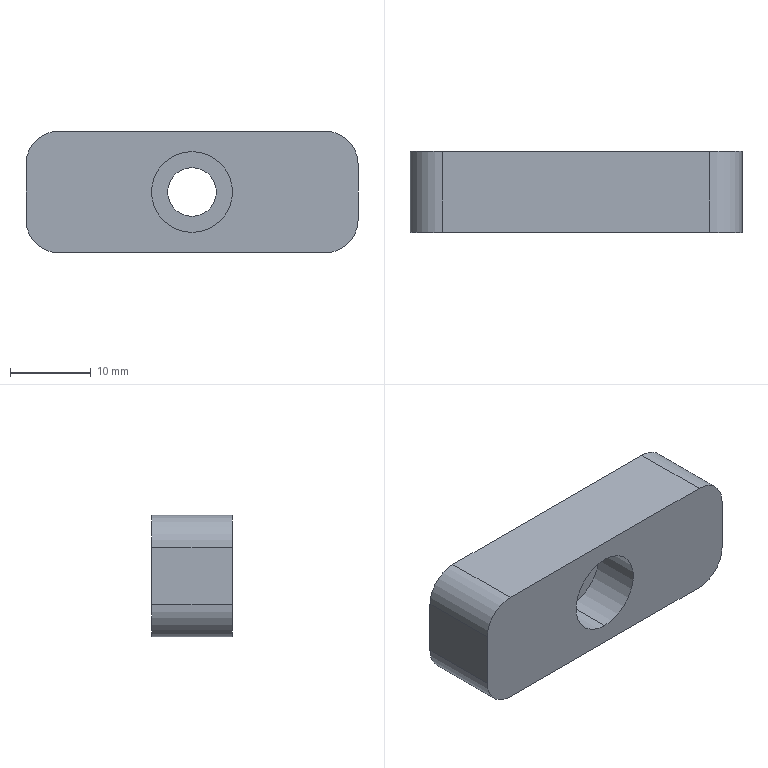Part | STEP file | 1 solid | 15 faces | box 41 x 10 x 15 mm | volume 5428 mm3 | cylinder 8 | plane 7 | commonest cylinder face diameters 8 x4 6 x2 10 x2
STEP:
#1=CARTESIAN_POINT('',(0.,0.,0.));
#2=DIRECTION('',(0.,0.,1.));
#3=DIRECTION('',(1.,0.,0.));
#4=AXIS2_PLACEMENT_3D('',#1,#2,#3);
#5=CARTESIAN_POINT('',(-27.135,-50.,198.714));
#6=VERTEX_POINT('',#5);
#7=CARTESIAN_POINT('',(-27.135,-44.,198.714));
#8=VERTEX_POINT('',#7);
#9=CARTESIAN_POINT('',(-27.135,-50.,198.714));
#10=DIRECTION('',(0.,1.,0.));
#11=VECTOR('',#10,1.);
#12=LINE('',#9,#11);
#13=CARTESIAN_POINT('',(-27.135,-50.,193.714));
#14=DIRECTION('',(0.,1.,0.));
#15=DIRECTION('',(0.,0.,1.));
#16=AXIS2_PLACEMENT_3D('',#13,#14,#15);
#17=CYLINDRICAL_SURFACE('',#16,5.);
#18=CARTESIAN_POINT('',(6.283,0.));
#19=DIRECTION('',(0.,1.));
#20=VECTOR('',#19,1.);
#21=LINE('',#18,#20);
#22=(GEOMETRIC_REPRESENTATION_CONTEXT(2)PARAMETRIC_REPRESENTATION_CONTEXT()REPRESENTATION_CONTEXT('',''));
#23=DEFINITIONAL_REPRESENTATION('',(#21),#22);
#24=PCURVE('',#17,#23);
#25=CARTESIAN_POINT('',(-27.135,-50.,193.714));
#26=DIRECTION('',(0.,1.,0.));
#27=DIRECTION('',(0.,0.,1.));
#28=AXIS2_PLACEMENT_3D('',#25,#26,#27);
#29=CYLINDRICAL_SURFACE('',#28,5.);
#30=CARTESIAN_POINT('',(0.,0.));
#31=DIRECTION('',(0.,1.));
#32=VECTOR('',#31,1.);
#33=LINE('',#30,#32);
#34=(GEOMETRIC_REPRESENTATION_CONTEXT(2)PARAMETRIC_REPRESENTATION_CONTEXT()REPRESENTATION_CONTEXT('',''));
#35=DEFINITIONAL_REPRESENTATION('',(#33),#34);
#36=PCURVE('',#29,#35);
#37=SURFACE_CURVE('',#12,(#24,#36),.PCURVE_S1.);
#38=EDGE_CURVE('',#6,#8,#37,.T.);
#39=ORIENTED_EDGE('',*,*,#38,.T.);
#40=CARTESIAN_POINT('',(-27.135,-44.,188.714));
#41=VERTEX_POINT('',#40);
#42=CARTESIAN_POINT('',(-27.135,-44.,193.714));
#43=DIRECTION('',(0.,1.,0.));
#44=DIRECTION('',(0.,0.,-1.));
#45=AXIS2_PLACEMENT_3D('',#42,#43,#44);
#46=CIRCLE('',#45,5.);
#47=CARTESIAN_POINT('',(3.142,6.));
#48=DIRECTION('',(1.,0.));
#49=VECTOR('',#48,1.);
#50=LINE('',#47,#49);
#51=(GEOMETRIC_REPRESENTATION_CONTEXT(2)PARAMETRIC_REPRESENTATION_CONTEXT()REPRESENTATION_CONTEXT('',''));
#52=DEFINITIONAL_REPRESENTATION('',(#50),#51);
#53=PCURVE('',#17,#52);
#54=CARTESIAN_POINT('',(-27.135,-44.,193.714));
#55=DIRECTION('',(0.,1.,0.));
#56=DIRECTION('',(0.,0.,1.));
#57=AXIS2_PLACEMENT_3D('',#54,#55,#56);
#58=PLANE('',#57);
#59=CARTESIAN_POINT('',(0.,0.));
#60=DIRECTION('',(-1.,0.));
#61=AXIS2_PLACEMENT_2D('',#59,#60);
#62=CIRCLE('',#61,5.);
#63=(GEOMETRIC_REPRESENTATION_CONTEXT(2)PARAMETRIC_REPRESENTATION_CONTEXT()REPRESENTATION_CONTEXT('',''));
#64=DEFINITIONAL_REPRESENTATION('',(#62),#63);
#65=PCURVE('',#58,#64);
#66=SURFACE_CURVE('',#46,(#53,#65),.PCURVE_S1.);
#67=EDGE_CURVE('',#41,#8,#66,.T.);
#68=ORIENTED_EDGE('',*,*,#67,.F.);
#69=CARTESIAN_POINT('',(-27.135,-50.,188.714));
#70=VERTEX_POINT('',#69);
#71=CARTESIAN_POINT('',(-27.135,-50.,188.714));
#72=DIRECTION('',(0.,1.,0.));
#73=VECTOR('',#72,1.);
#74=LINE('',#71,#73);
#75=CARTESIAN_POINT('',(3.142,0.));
#76=DIRECTION('',(0.,1.));
#77=VECTOR('',#76,1.);
#78=LINE('',#75,#77);
#79=(GEOMETRIC_REPRESENTATION_CONTEXT(2)PARAMETRIC_REPRESENTATION_CONTEXT()REPRESENTATION_CONTEXT('',''));
#80=DEFINITIONAL_REPRESENTATION('',(#78),#79);
#81=PCURVE('',#17,#80);
#82=CARTESIAN_POINT('',(3.142,0.));
#83=DIRECTION('',(0.,1.));
#84=VECTOR('',#83,1.);
#85=LINE('',#82,#84);
#86=(GEOMETRIC_REPRESENTATION_CONTEXT(2)PARAMETRIC_REPRESENTATION_CONTEXT()REPRESENTATION_CONTEXT('',''));
#87=DEFINITIONAL_REPRESENTATION('',(#85),#86);
#88=PCURVE('',#29,#87);
#89=SURFACE_CURVE('',#74,(#81,#88),.PCURVE_S1.);
#90=EDGE_CURVE('',#70,#41,#89,.T.);
#91=ORIENTED_EDGE('',*,*,#90,.F.);
#92=CARTESIAN_POINT('',(-27.135,-50.,193.714));
#93=DIRECTION('',(0.,-1.,0.));
#94=DIRECTION('',(0.,0.,1.));
#95=AXIS2_PLACEMENT_3D('',#92,#93,#94);
#96=CIRCLE('',#95,5.);
#97=CARTESIAN_POINT('',(6.283,0.));
#98=DIRECTION('',(-1.,0.));
#99=VECTOR('',#98,1.);
#100=LINE('',#97,#99);
#101=(GEOMETRIC_REPRESENTATION_CONTEXT(2)PARAMETRIC_REPRESENTATION_CONTEXT()REPRESENTATION_CONTEXT('',''));
#102=DEFINITIONAL_REPRESENTATION('',(#100),#101);
#103=PCURVE('',#17,#102);
#104=CARTESIAN_POINT('',(-27.135,-50.,189.963));
#105=DIRECTION('',(0.,-1.,0.));
#106=DIRECTION('',(0.,0.,-1.));
#107=AXIS2_PLACEMENT_3D('',#104,#105,#106);
#108=PLANE('',#107);
#109=CARTESIAN_POINT('',(-3.751,0.));
#110=DIRECTION('',(-1.,0.));
#111=AXIS2_PLACEMENT_2D('',#109,#110);
#112=CIRCLE('',#111,5.);
#113=(GEOMETRIC_REPRESENTATION_CONTEXT(2)PARAMETRIC_REPRESENTATION_CONTEXT()REPRESENTATION_CONTEXT('',''));
#114=DEFINITIONAL_REPRESENTATION('',(#112),#113);
#115=PCURVE('',#108,#114);
#116=SURFACE_CURVE('',#96,(#103,#115),.PCURVE_S1.);
#117=EDGE_CURVE('',#6,#70,#116,.T.);
#118=ORIENTED_EDGE('',*,*,#117,.F.);
#119=EDGE_LOOP('',(#39,#68,#91,#118));
#120=FACE_BOUND('',#119,.F.);
#121=ADVANCED_FACE('',(#120),#17,.F.);
#122=CARTESIAN_POINT('',(-27.135,-44.,196.714));
#123=VERTEX_POINT('',#122);
#124=CARTESIAN_POINT('',(-27.135,-40.,196.714));
#125=VERTEX_POINT('',#124);
#126=CARTESIAN_POINT('',(-27.135,-50.,196.714));
#127=DIRECTION('',(0.,1.,0.));
#128=VECTOR('',#127,1.);
#129=LINE('',#126,#128);
#130=CARTESIAN_POINT('',(-27.135,-50.,193.714));
#131=DIRECTION('',(0.,1.,0.));
#132=DIRECTION('',(0.,0.,1.));
#133=AXIS2_PLACEMENT_3D('',#130,#131,#132);
#134=CYLINDRICAL_SURFACE('',#133,3.);
#135=CARTESIAN_POINT('',(6.283,0.));
#136=DIRECTION('',(0.,1.));
#137=VECTOR('',#136,1.);
#138=LINE('',#135,#137);
#139=(GEOMETRIC_REPRESENTATION_CONTEXT(2)PARAMETRIC_REPRESENTATION_CONTEXT()REPRESENTATION_CONTEXT('',''));
#140=DEFINITIONAL_REPRESENTATION('',(#138),#139);
#141=PCURVE('',#134,#140);
#142=CARTESIAN_POINT('',(-27.135,-50.,193.714));
#143=DIRECTION('',(0.,1.,0.));
#144=DIRECTION('',(0.,0.,1.));
#145=AXIS2_PLACEMENT_3D('',#142,#143,#144);
#146=CYLINDRICAL_SURFACE('',#145,3.);
#147=CARTESIAN_POINT('',(0.,0.));
#148=DIRECTION('',(0.,1.));
#149=VECTOR('',#148,1.);
#150=LINE('',#147,#149);
#151=(GEOMETRIC_REPRESENTATION_CONTEXT(2)PARAMETRIC_REPRESENTATION_CONTEXT()REPRESENTATION_CONTEXT('',''));
#152=DEFINITIONAL_REPRESENTATION('',(#150),#151);
#153=PCURVE('',#146,#152);
#154=SURFACE_CURVE('',#129,(#141,#153),.PCURVE_S1.);
#155=EDGE_CURVE('',#123,#125,#154,.T.);
#156=ORIENTED_EDGE('',*,*,#155,.T.);
#157=CARTESIAN_POINT('',(-27.135,-40.,190.714));
#158=VERTEX_POINT('',#157);
#159=CARTESIAN_POINT('',(-27.135,-40.,193.714));
#160=DIRECTION('',(0.,1.,0.));
#161=DIRECTION('',(0.,0.,-1.));
#162=AXIS2_PLACEMENT_3D('',#159,#160,#161);
#163=CIRCLE('',#162,3.);
#164=CARTESIAN_POINT('',(3.142,10.));
#165=DIRECTION('',(1.,0.));
#166=VECTOR('',#165,1.);
#167=LINE('',#164,#166);
#168=(GEOMETRIC_REPRESENTATION_CONTEXT(2)PARAMETRIC_REPRESENTATION_CONTEXT()REPRESENTATION_CONTEXT('',''));
#169=DEFINITIONAL_REPRESENTATION('',(#167),#168);
#170=PCURVE('',#134,#169);
#171=CARTESIAN_POINT('',(-27.135,-40.,193.714));
#172=DIRECTION('',(0.,-1.,0.));
#173=DIRECTION('',(0.,0.,-1.));
#174=AXIS2_PLACEMENT_3D('',#171,#172,#173);
#175=PLANE('',#174);
#176=CARTESIAN_POINT('',(3.,0.));
#177=CARTESIAN_POINT('',(3.,-5.196));
#178=CARTESIAN_POINT('',(-1.5,-2.598));
#179=CARTESIAN_POINT('',(-6.,0.));
#180=CARTESIAN_POINT('',(-1.5,2.598));
#181=CARTESIAN_POINT('',(3.,5.196));
#182=CARTESIAN_POINT('',(3.,0.));
#183=(BOUNDED_CURVE()B_SPLINE_CURVE(2,(#176,#177,#178,#179,#180,#181,#182),.UNSPECIFIED.,.T.,.F.)B_SPLINE_CURVE_WITH_KNOTS((1,2,2,2,2,1),(-2.094,0.,2.094,4.189,6.283,8.378),.UNSPECIFIED.)CURVE()GEOMETRIC_REPRESENTATION_ITEM()RATIONAL_B_SPLINE_CURVE((1.,0.5,1.,0.5,1.,0.5,1.))REPRESENTATION_ITEM(''));
#184=(GEOMETRIC_REPRESENTATION_CONTEXT(2)PARAMETRIC_REPRESENTATION_CONTEXT()REPRESENTATION_CONTEXT('',''));
#185=DEFINITIONAL_REPRESENTATION('',(#183),#184);
#186=PCURVE('',#175,#185);
#187=SURFACE_CURVE('',#163,(#170,#186),.PCURVE_S1.);
#188=EDGE_CURVE('',#158,#125,#187,.T.);
#189=ORIENTED_EDGE('',*,*,#188,.F.);
#190=CARTESIAN_POINT('',(-27.135,-44.,190.714));
#191=VERTEX_POINT('',#190);
#192=CARTESIAN_POINT('',(-27.135,-50.,190.714));
#193=DIRECTION('',(0.,1.,0.));
#194=VECTOR('',#193,1.);
#195=LINE('',#192,#194);
#196=CARTESIAN_POINT('',(3.142,0.));
#197=DIRECTION('',(0.,1.));
#198=VECTOR('',#197,1.);
#199=LINE('',#196,#198);
#200=(GEOMETRIC_REPRESENTATION_CONTEXT(2)PARAMETRIC_REPRESENTATION_CONTEXT()REPRESENTATION_CONTEXT('',''));
#201=DEFINITIONAL_REPRESENTATION('',(#199),#200);
#202=PCURVE('',#134,#201);
#203=CARTESIAN_POINT('',(3.142,0.));
#204=DIRECTION('',(0.,1.));
#205=VECTOR('',#204,1.);
#206=LINE('',#203,#205);
#207=(GEOMETRIC_REPRESENTATION_CONTEXT(2)PARAMETRIC_REPRESENTATION_CONTEXT()REPRESENTATION_CONTEXT('',''));
#208=DEFINITIONAL_REPRESENTATION('',(#206),#207);
#209=PCURVE('',#146,#208);
#210=SURFACE_CURVE('',#195,(#202,#209),.PCURVE_S1.);
#211=EDGE_CURVE('',#191,#158,#210,.T.);
#212=ORIENTED_EDGE('',*,*,#211,.F.);
#213=CARTESIAN_POINT('',(-27.135,-44.,193.714));
#214=DIRECTION('',(0.,1.,0.));
#215=DIRECTION('',(0.,0.,1.));
#216=AXIS2_PLACEMENT_3D('',#213,#214,#215);
#217=CIRCLE('',#216,3.);
#218=CARTESIAN_POINT('',(0.,6.));
#219=DIRECTION('',(1.,0.));
#220=VECTOR('',#219,1.);
#221=LINE('',#218,#220);
#222=(GEOMETRIC_REPRESENTATION_CONTEXT(2)PARAMETRIC_REPRESENTATION_CONTEXT()REPRESENTATION_CONTEXT('',''));
#223=DEFINITIONAL_REPRESENTATION('',(#221),#222);
#224=PCURVE('',#134,#223);
#225=CARTESIAN_POINT('',(0.,0.));
#226=DIRECTION('',(1.,0.));
#227=AXIS2_PLACEMENT_2D('',#225,#226);
#228=CIRCLE('',#227,3.);
#229=(GEOMETRIC_REPRESENTATION_CONTEXT(2)PARAMETRIC_REPRESENTATION_CONTEXT()REPRESENTATION_CONTEXT('',''));
#230=DEFINITIONAL_REPRESENTATION('',(#228),#229);
#231=PCURVE('',#58,#230);
#232=SURFACE_CURVE('',#217,(#224,#231),.PCURVE_S1.);
#233=EDGE_CURVE('',#191,#123,#232,.T.);
#234=ORIENTED_EDGE('',*,*,#233,.T.);
#235=EDGE_LOOP('',(#156,#189,#212,#234));
#236=FACE_BOUND('',#235,.F.);
#237=ADVANCED_FACE('',(#236),#134,.F.);
#238=CARTESIAN_POINT('',(-43.635,-40.,201.214));
#239=VERTEX_POINT('',#238);
#240=CARTESIAN_POINT('',(-10.635,-40.,201.214));
#241=VERTEX_POINT('',#240);
#242=CARTESIAN_POINT('',(-27.135,-40.,201.214));
#243=DIRECTION('',(1.,0.,0.));
#244=VECTOR('',#243,1.);
#245=LINE('',#242,#244);
#246=CARTESIAN_POINT('',(-47.635,-40.,201.214));
#247=DIRECTION('',(0.,0.,1.));
#248=DIRECTION('',(-1.,0.,0.));
#249=AXIS2_PLACEMENT_3D('',#246,#247,#248);
#250=PLANE('',#249);
#251=CARTESIAN_POINT('',(-20.5,0.));
#252=DIRECTION('',(-1.,0.));
#253=VECTOR('',#252,1.);
#254=LINE('',#251,#253);
#255=(GEOMETRIC_REPRESENTATION_CONTEXT(2)PARAMETRIC_REPRESENTATION_CONTEXT()REPRESENTATION_CONTEXT('',''));
#256=DEFINITIONAL_REPRESENTATION('',(#254),#255);
#257=PCURVE('',#250,#256);
#258=CARTESIAN_POINT('',(-7.5,0.));
#259=DIRECTION('',(0.,1.));
#260=VECTOR('',#259,1.);
#261=LINE('',#258,#260);
#262=(GEOMETRIC_REPRESENTATION_CONTEXT(2)PARAMETRIC_REPRESENTATION_CONTEXT()REPRESENTATION_CONTEXT('',''));
#263=DEFINITIONAL_REPRESENTATION('',(#261),#262);
#264=PCURVE('',#175,#263);
#265=SURFACE_CURVE('',#245,(#257,#264),.PCURVE_S1.);
#266=EDGE_CURVE('',#239,#241,#265,.T.);
#267=ORIENTED_EDGE('',*,*,#266,.F.);
#268=CARTESIAN_POINT('',(-43.635,-50.,201.214));
#269=VERTEX_POINT('',#268);
#270=CARTESIAN_POINT('',(-43.635,-40.,201.214));
#271=DIRECTION('',(0.,1.,0.));
#272=VECTOR('',#271,1.);
#273=LINE('',#270,#272);
#274=CARTESIAN_POINT('',(-4.,0.));
#275=DIRECTION('',(0.,-1.));
#276=VECTOR('',#275,1.);
#277=LINE('',#274,#276);
#278=(GEOMETRIC_REPRESENTATION_CONTEXT(2)PARAMETRIC_REPRESENTATION_CONTEXT()REPRESENTATION_CONTEXT('',''));
#279=DEFINITIONAL_REPRESENTATION('',(#277),#278);
#280=PCURVE('',#250,#279);
#281=CARTESIAN_POINT('',(-43.635,-50.,197.214));
#282=DIRECTION('',(0.,-1.,0.));
#283=DIRECTION('',(0.,0.,-1.));
#284=AXIS2_PLACEMENT_3D('',#281,#282,#283);
#285=CYLINDRICAL_SURFACE('',#284,4.);
#286=CARTESIAN_POINT('',(3.142,-10.));
#287=DIRECTION('',(0.,-1.));
#288=VECTOR('',#287,1.);
#289=LINE('',#286,#288);
#290=(GEOMETRIC_REPRESENTATION_CONTEXT(2)PARAMETRIC_REPRESENTATION_CONTEXT()REPRESENTATION_CONTEXT('',''));
#291=DEFINITIONAL_REPRESENTATION('',(#289),#290);
#292=PCURVE('',#285,#291);
#293=SURFACE_CURVE('',#273,(#280,#292),.PCURVE_S1.);
#294=EDGE_CURVE('',#269,#239,#293,.T.);
#295=ORIENTED_EDGE('',*,*,#294,.F.);
#296=CARTESIAN_POINT('',(-10.635,-50.,201.214));
#297=VERTEX_POINT('',#296);
#298=CARTESIAN_POINT('',(-27.135,-50.,201.214));
#299=DIRECTION('',(1.,0.,0.));
#300=VECTOR('',#299,1.);
#301=LINE('',#298,#300);
#302=CARTESIAN_POINT('',(-20.5,10.));
#303=DIRECTION('',(-1.,0.));
#304=VECTOR('',#303,1.);
#305=LINE('',#302,#304);
#306=(GEOMETRIC_REPRESENTATION_CONTEXT(2)PARAMETRIC_REPRESENTATION_CONTEXT()REPRESENTATION_CONTEXT('',''));
#307=DEFINITIONAL_REPRESENTATION('',(#305),#306);
#308=PCURVE('',#250,#307);
#309=CARTESIAN_POINT('',(-11.251,0.));
#310=DIRECTION('',(0.,1.));
#311=VECTOR('',#310,1.);
#312=LINE('',#309,#311);
#313=(GEOMETRIC_REPRESENTATION_CONTEXT(2)PARAMETRIC_REPRESENTATION_CONTEXT()REPRESENTATION_CONTEXT('',''));
#314=DEFINITIONAL_REPRESENTATION('',(#312),#313);
#315=PCURVE('',#108,#314);
#316=SURFACE_CURVE('',#301,(#308,#315),.PCURVE_S1.);
#317=EDGE_CURVE('',#269,#297,#316,.T.);
#318=ORIENTED_EDGE('',*,*,#317,.T.);
#319=CARTESIAN_POINT('',(-10.635,-50.,201.214));
#320=DIRECTION('',(0.,-1.,0.));
#321=VECTOR('',#320,1.);
#322=LINE('',#319,#321);
#323=CARTESIAN_POINT('',(-37.,10.));
#324=DIRECTION('',(0.,1.));
#325=VECTOR('',#324,1.);
#326=LINE('',#323,#325);
#327=(GEOMETRIC_REPRESENTATION_CONTEXT(2)PARAMETRIC_REPRESENTATION_CONTEXT()REPRESENTATION_CONTEXT('',''));
#328=DEFINITIONAL_REPRESENTATION('',(#326),#327);
#329=PCURVE('',#250,#328);
#330=CARTESIAN_POINT('',(-10.635,-40.,197.214));
#331=DIRECTION('',(0.,1.,0.));
#332=DIRECTION('',(0.,0.,1.));
#333=AXIS2_PLACEMENT_3D('',#330,#331,#332);
#334=CYLINDRICAL_SURFACE('',#333,4.);
#335=CARTESIAN_POINT('',(0.,-10.));
#336=DIRECTION('',(0.,-1.));
#337=VECTOR('',#336,1.);
#338=LINE('',#335,#337);
#339=(GEOMETRIC_REPRESENTATION_CONTEXT(2)PARAMETRIC_REPRESENTATION_CONTEXT()REPRESENTATION_CONTEXT('',''));
#340=DEFINITIONAL_REPRESENTATION('',(#338),#339);
#341=PCURVE('',#334,#340);
#342=SURFACE_CURVE('',#322,(#329,#341),.PCURVE_S1.);
#343=EDGE_CURVE('',#241,#297,#342,.T.);
#344=ORIENTED_EDGE('',*,*,#343,.F.);
#345=EDGE_LOOP('',(#267,#295,#318,#344));
#346=FACE_BOUND('',#345,.T.);
#347=ADVANCED_FACE('',(#346),#250,.T.);
#348=CARTESIAN_POINT('',(-6.635,-50.,190.214));
#349=VERTEX_POINT('',#348);
#350=CARTESIAN_POINT('',(-6.635,-50.,197.214));
#351=VERTEX_POINT('',#350);
#352=CARTESIAN_POINT('',(-6.635,-50.,189.963));
#353=DIRECTION('',(0.,0.,1.));
#354=VECTOR('',#353,1.);
#355=LINE('',#352,#354);
#356=CARTESIAN_POINT('',(-6.635,-50.,202.465));
#357=DIRECTION('',(-1.,0.,0.));
#358=DIRECTION('',(0.,0.,-1.));
#359=AXIS2_PLACEMENT_3D('',#356,#357,#358);
#360=PLANE('',#359);
#361=CARTESIAN_POINT('',(12.502,0.));
#362=DIRECTION('',(-1.,0.));
#363=VECTOR('',#362,1.);
#364=LINE('',#361,#363);
#365=(GEOMETRIC_REPRESENTATION_CONTEXT(2)PARAMETRIC_REPRESENTATION_CONTEXT()REPRESENTATION_CONTEXT('',''));
#366=DEFINITIONAL_REPRESENTATION('',(#364),#365);
#367=PCURVE('',#360,#366);
#368=CARTESIAN_POINT('',(0.,20.5));
#369=DIRECTION('',(-1.,0.));
#370=VECTOR('',#369,1.);
#371=LINE('',#368,#370);
#372=(GEOMETRIC_REPRESENTATION_CONTEXT(2)PARAMETRIC_REPRESENTATION_CONTEXT()REPRESENTATION_CONTEXT('',''));
#373=DEFINITIONAL_REPRESENTATION('',(#371),#372);
#374=PCURVE('',#108,#373);
#375=SURFACE_CURVE('',#355,(#367,#374),.PCURVE_S1.);
#376=EDGE_CURVE('',#349,#351,#375,.T.);
#377=ORIENTED_EDGE('',*,*,#376,.F.);
#378=CARTESIAN_POINT('',(-6.635,-40.,190.214));
#379=VERTEX_POINT('',#378);
#380=CARTESIAN_POINT('',(-6.635,-50.,190.214));
#381=DIRECTION('',(0.,-1.,0.));
#382=VECTOR('',#381,1.);
#383=LINE('',#380,#382);
#384=CARTESIAN_POINT('',(12.251,0.));
#385=DIRECTION('',(0.,1.));
#386=VECTOR('',#385,1.);
#387=LINE('',#384,#386);
#388=(GEOMETRIC_REPRESENTATION_CONTEXT(2)PARAMETRIC_REPRESENTATION_CONTEXT()REPRESENTATION_CONTEXT('',''));
#389=DEFINITIONAL_REPRESENTATION('',(#387),#388);
#390=PCURVE('',#360,#389);
#391=CARTESIAN_POINT('',(-10.635,-50.,190.214));
#392=DIRECTION('',(0.,-1.,0.));
#393=DIRECTION('',(0.,0.,-1.));
#394=AXIS2_PLACEMENT_3D('',#391,#392,#393);
#395=CYLINDRICAL_SURFACE('',#394,4.);
#396=CARTESIAN_POINT('',(1.571,0.));
#397=DIRECTION('',(0.,1.));
#398=VECTOR('',#397,1.);
#399=LINE('',#396,#398);
#400=(GEOMETRIC_REPRESENTATION_CONTEXT(2)PARAMETRIC_REPRESENTATION_CONTEXT()REPRESENTATION_CONTEXT('',''));
#401=DEFINITIONAL_REPRESENTATION('',(#399),#400);
#402=PCURVE('',#395,#401);
#403=SURFACE_CURVE('',#383,(#390,#402),.PCURVE_S1.);
#404=EDGE_CURVE('',#379,#349,#403,.T.);
#405=ORIENTED_EDGE('',*,*,#404,.F.);
#406=CARTESIAN_POINT('',(-6.635,-40.,197.214));
#407=VERTEX_POINT('',#406);
#408=CARTESIAN_POINT('',(-6.635,-40.,193.714));
#409=DIRECTION('',(0.,0.,1.));
#410=VECTOR('',#409,1.);
#411=LINE('',#408,#410);
#412=CARTESIAN_POINT('',(8.751,-10.));
#413=DIRECTION('',(-1.,0.));
#414=VECTOR('',#413,1.);
#415=LINE('',#412,#414);
#416=(GEOMETRIC_REPRESENTATION_CONTEXT(2)PARAMETRIC_REPRESENTATION_CONTEXT()REPRESENTATION_CONTEXT('',''));
#417=DEFINITIONAL_REPRESENTATION('',(#415),#416);
#418=PCURVE('',#360,#417);
#419=CARTESIAN_POINT('',(0.,20.5));
#420=DIRECTION('',(-1.,0.));
#421=VECTOR('',#420,1.);
#422=LINE('',#419,#421);
#423=(GEOMETRIC_REPRESENTATION_CONTEXT(2)PARAMETRIC_REPRESENTATION_CONTEXT()REPRESENTATION_CONTEXT('',''));
#424=DEFINITIONAL_REPRESENTATION('',(#422),#423);
#425=PCURVE('',#175,#424);
#426=SURFACE_CURVE('',#411,(#418,#425),.PCURVE_S1.);
#427=EDGE_CURVE('',#379,#407,#426,.T.);
#428=ORIENTED_EDGE('',*,*,#427,.T.);
#429=CARTESIAN_POINT('',(-6.635,-40.,197.214));
#430=DIRECTION('',(0.,1.,0.));
#431=VECTOR('',#430,1.);
#432=LINE('',#429,#431);
#433=CARTESIAN_POINT('',(5.251,-10.));
#434=DIRECTION('',(0.,-1.));
#435=VECTOR('',#434,1.);
#436=LINE('',#433,#435);
#437=(GEOMETRIC_REPRESENTATION_CONTEXT(2)PARAMETRIC_REPRESENTATION_CONTEXT()REPRESENTATION_CONTEXT('',''));
#438=DEFINITIONAL_REPRESENTATION('',(#436),#437);
#439=PCURVE('',#360,#438);
#440=CARTESIAN_POINT('',(1.571,0.));
#441=DIRECTION('',(0.,1.));
#442=VECTOR('',#441,1.);
#443=LINE('',#440,#442);
#444=(GEOMETRIC_REPRESENTATION_CONTEXT(2)PARAMETRIC_REPRESENTATION_CONTEXT()REPRESENTATION_CONTEXT('',''));
#445=DEFINITIONAL_REPRESENTATION('',(#443),#444);
#446=PCURVE('',#334,#445);
#447=SURFACE_CURVE('',#432,(#439,#446),.PCURVE_S1.);
#448=EDGE_CURVE('',#351,#407,#447,.T.);
#449=ORIENTED_EDGE('',*,*,#448,.F.);
#450=EDGE_LOOP('',(#377,#405,#428,#449));
#451=FACE_BOUND('',#450,.T.);
#452=ADVANCED_FACE('',(#451),#360,.F.);
#453=ORIENTED_EDGE('',*,*,#117,.F.);
#454=CARTESIAN_POINT('',(-27.135,-50.,193.714));
#455=DIRECTION('',(0.,-1.,0.));
#456=DIRECTION('',(0.,0.,1.));
#457=AXIS2_PLACEMENT_3D('',#454,#455,#456);
#458=CIRCLE('',#457,5.);
#459=CARTESIAN_POINT('',(-3.751,0.));
#460=DIRECTION('',(-1.,0.));
#461=AXIS2_PLACEMENT_2D('',#459,#460);
#462=CIRCLE('',#461,5.);
#463=(GEOMETRIC_REPRESENTATION_CONTEXT(2)PARAMETRIC_REPRESENTATION_CONTEXT()REPRESENTATION_CONTEXT('',''));
#464=DEFINITIONAL_REPRESENTATION('',(#462),#463);
#465=PCURVE('',#108,#464);
#466=CARTESIAN_POINT('',(6.283,0.));
#467=DIRECTION('',(-1.,0.));
#468=VECTOR('',#467,1.);
#469=LINE('',#466,#468);
#470=(GEOMETRIC_REPRESENTATION_CONTEXT(2)PARAMETRIC_REPRESENTATION_CONTEXT()REPRESENTATION_CONTEXT('',''));
#471=DEFINITIONAL_REPRESENTATION('',(#469),#470);
#472=PCURVE('',#29,#471);
#473=SURFACE_CURVE('',#458,(#465,#472),.PCURVE_S1.);
#474=EDGE_CURVE('',#70,#6,#473,.T.);
#475=ORIENTED_EDGE('',*,*,#474,.F.);
#476=EDGE_LOOP('',(#453,#475));
#477=FACE_BOUND('',#476,.T.);
#478=ORIENTED_EDGE('',*,*,#317,.F.);
#479=CARTESIAN_POINT('',(-47.635,-50.,197.214));
#480=VERTEX_POINT('',#479);
#481=CARTESIAN_POINT('',(-43.635,-50.,197.214));
#482=DIRECTION('',(0.,1.,0.));
#483=DIRECTION('',(0.,0.,-1.));
#484=AXIS2_PLACEMENT_3D('',#481,#482,#483);
#485=CIRCLE('',#484,4.);
#486=CARTESIAN_POINT('',(-3.251,-16.5));
#487=CARTESIAN_POINT('',(-3.251,-23.428));
#488=CARTESIAN_POINT('',(-9.251,-19.964));
#489=CARTESIAN_POINT('',(-15.251,-16.5));
#490=CARTESIAN_POINT('',(-9.251,-13.036));
#491=CARTESIAN_POINT('',(-3.251,-9.572));
#492=CARTESIAN_POINT('',(-3.251,-16.5));
#493=(BOUNDED_CURVE()B_SPLINE_CURVE(2,(#486,#487,#488,#489,#490,#491,#492),.UNSPECIFIED.,.T.,.F.)B_SPLINE_CURVE_WITH_KNOTS((1,2,2,2,2,1),(-2.094,0.,2.094,4.189,6.283,8.378),.UNSPECIFIED.)CURVE()GEOMETRIC_REPRESENTATION_ITEM()RATIONAL_B_SPLINE_CURVE((1.,0.5,1.,0.5,1.,0.5,1.))REPRESENTATION_ITEM(''));
#494=(GEOMETRIC_REPRESENTATION_CONTEXT(2)PARAMETRIC_REPRESENTATION_CONTEXT()REPRESENTATION_CONTEXT('',''));
#495=DEFINITIONAL_REPRESENTATION('',(#493),#494);
#496=PCURVE('',#108,#495);
#497=CARTESIAN_POINT('',(6.283,0.));
#498=DIRECTION('',(-1.,0.));
#499=VECTOR('',#498,1.);
#500=LINE('',#497,#499);
#501=(GEOMETRIC_REPRESENTATION_CONTEXT(2)PARAMETRIC_REPRESENTATION_CONTEXT()REPRESENTATION_CONTEXT('',''));
#502=DEFINITIONAL_REPRESENTATION('',(#500),#501);
#503=PCURVE('',#285,#502);
#504=SURFACE_CURVE('',#485,(#496,#503),.PCURVE_S1.);
#505=EDGE_CURVE('',#480,#269,#504,.T.);
#506=ORIENTED_EDGE('',*,*,#505,.F.);
#507=CARTESIAN_POINT('',(-47.635,-50.,190.214));
#508=VERTEX_POINT('',#507);
#509=CARTESIAN_POINT('',(-47.635,-50.,189.963));
#510=DIRECTION('',(0.,0.,1.));
#511=VECTOR('',#510,1.);
#512=LINE('',#509,#511);
#513=CARTESIAN_POINT('',(0.,-20.5));
#514=DIRECTION('',(-1.,0.));
#515=VECTOR('',#514,1.);
#516=LINE('',#513,#515);
#517=(GEOMETRIC_REPRESENTATION_CONTEXT(2)PARAMETRIC_REPRESENTATION_CONTEXT()REPRESENTATION_CONTEXT('',''));
#518=DEFINITIONAL_REPRESENTATION('',(#516),#517);
#519=PCURVE('',#108,#518);
#520=CARTESIAN_POINT('',(-47.635,-50.,202.465));
#521=DIRECTION('',(-1.,0.,0.));
#522=DIRECTION('',(0.,0.,-1.));
#523=AXIS2_PLACEMENT_3D('',#520,#521,#522);
#524=PLANE('',#523);
#525=CARTESIAN_POINT('',(12.502,0.));
#526=DIRECTION('',(-1.,0.));
#527=VECTOR('',#526,1.);
#528=LINE('',#525,#527);
#529=(GEOMETRIC_REPRESENTATION_CONTEXT(2)PARAMETRIC_REPRESENTATION_CONTEXT()REPRESENTATION_CONTEXT('',''));
#530=DEFINITIONAL_REPRESENTATION('',(#528),#529);
#531=PCURVE('',#524,#530);
#532=SURFACE_CURVE('',#512,(#519,#531),.PCURVE_S1.);
#533=EDGE_CURVE('',#508,#480,#532,.T.);
#534=ORIENTED_EDGE('',*,*,#533,.F.);
#535=CARTESIAN_POINT('',(-43.635,-50.,186.214));
#536=VERTEX_POINT('',#535);
#537=CARTESIAN_POINT('',(-43.635,-50.,190.214));
#538=DIRECTION('',(0.,1.,0.));
#539=DIRECTION('',(0.,0.,-1.));
#540=AXIS2_PLACEMENT_3D('',#537,#538,#539);
#541=CIRCLE('',#540,4.);
#542=CARTESIAN_POINT('',(3.749,-16.5));
#543=CARTESIAN_POINT('',(3.749,-23.428));
#544=CARTESIAN_POINT('',(-2.251,-19.964));
#545=CARTESIAN_POINT('',(-8.251,-16.5));
#546=CARTESIAN_POINT('',(-2.251,-13.036));
#547=CARTESIAN_POINT('',(3.749,-9.572));
#548=CARTESIAN_POINT('',(3.749,-16.5));
#549=(BOUNDED_CURVE()B_SPLINE_CURVE(2,(#542,#543,#544,#545,#546,#547,#548),.UNSPECIFIED.,.T.,.F.)B_SPLINE_CURVE_WITH_KNOTS((1,2,2,2,2,1),(-2.094,0.,2.094,4.189,6.283,8.378),.UNSPECIFIED.)CURVE()GEOMETRIC_REPRESENTATION_ITEM()RATIONAL_B_SPLINE_CURVE((1.,0.5,1.,0.5,1.,0.5,1.))REPRESENTATION_ITEM(''));
#550=(GEOMETRIC_REPRESENTATION_CONTEXT(2)PARAMETRIC_REPRESENTATION_CONTEXT()REPRESENTATION_CONTEXT('',''));
#551=DEFINITIONAL_REPRESENTATION('',(#549),#550);
#552=PCURVE('',#108,#551);
#553=CARTESIAN_POINT('',(-43.635,-40.,190.214));
#554=DIRECTION('',(0.,1.,0.));
#555=DIRECTION('',(0.,0.,1.));
#556=AXIS2_PLACEMENT_3D('',#553,#554,#555);
#557=CYLINDRICAL_SURFACE('',#556,4.);
#558=CARTESIAN_POINT('',(3.142,-10.));
#559=DIRECTION('',(1.,0.));
#560=VECTOR('',#559,1.);
#561=LINE('',#558,#560);
#562=(GEOMETRIC_REPRESENTATION_CONTEXT(2)PARAMETRIC_REPRESENTATION_CONTEXT()REPRESENTATION_CONTEXT('',''));
#563=DEFINITIONAL_REPRESENTATION('',(#561),#562);
#564=PCURVE('',#557,#563);
#565=SURFACE_CURVE('',#541,(#552,#564),.PCURVE_S1.);
#566=EDGE_CURVE('',#536,#508,#565,.T.);
#567=ORIENTED_EDGE('',*,*,#566,.F.);
#568=CARTESIAN_POINT('',(-10.635,-50.,186.214));
#569=VERTEX_POINT('',#568);
#570=CARTESIAN_POINT('',(-27.135,-50.,186.214));
#571=DIRECTION('',(1.,0.,0.));
#572=VECTOR('',#571,1.);
#573=LINE('',#570,#572);
#574=CARTESIAN_POINT('',(3.749,0.));
#575=DIRECTION('',(0.,1.));
#576=VECTOR('',#575,1.);
#577=LINE('',#574,#576);
#578=(GEOMETRIC_REPRESENTATION_CONTEXT(2)PARAMETRIC_REPRESENTATION_CONTEXT()REPRESENTATION_CONTEXT('',''));
#579=DEFINITIONAL_REPRESENTATION('',(#577),#578);
#580=PCURVE('',#108,#579);
#581=CARTESIAN_POINT('',(-47.635,-40.,186.214));
#582=DIRECTION('',(0.,0.,1.));
#583=DIRECTION('',(-1.,0.,0.));
#584=AXIS2_PLACEMENT_3D('',#581,#582,#583);
#585=PLANE('',#584);
#586=CARTESIAN_POINT('',(-20.5,10.));
#587=DIRECTION('',(-1.,0.));
#588=VECTOR('',#587,1.);
#589=LINE('',#586,#588);
#590=(GEOMETRIC_REPRESENTATION_CONTEXT(2)PARAMETRIC_REPRESENTATION_CONTEXT()REPRESENTATION_CONTEXT('',''));
#591=DEFINITIONAL_REPRESENTATION('',(#589),#590);
#592=PCURVE('',#585,#591);
#593=SURFACE_CURVE('',#573,(#580,#592),.PCURVE_S1.);
#594=EDGE_CURVE('',#536,#569,#593,.T.);
#595=ORIENTED_EDGE('',*,*,#594,.T.);
#596=CARTESIAN_POINT('',(-10.635,-50.,190.214));
#597=DIRECTION('',(0.,1.,0.));
#598=DIRECTION('',(0.,0.,-1.));
#599=AXIS2_PLACEMENT_3D('',#596,#597,#598);
#600=CIRCLE('',#599,4.);
#601=CARTESIAN_POINT('',(3.749,16.5));
#602=CARTESIAN_POINT('',(3.749,9.572));
#603=CARTESIAN_POINT('',(-2.251,13.036));
#604=CARTESIAN_POINT('',(-8.251,16.5));
#605=CARTESIAN_POINT('',(-2.251,19.964));
#606=CARTESIAN_POINT('',(3.749,23.428));
#607=CARTESIAN_POINT('',(3.749,16.5));
#608=(BOUNDED_CURVE()B_SPLINE_CURVE(2,(#601,#602,#603,#604,#605,#606,#607),.UNSPECIFIED.,.T.,.F.)B_SPLINE_CURVE_WITH_KNOTS((1,2,2,2,2,1),(-2.094,0.,2.094,4.189,6.283,8.378),.UNSPECIFIED.)CURVE()GEOMETRIC_REPRESENTATION_ITEM()RATIONAL_B_SPLINE_CURVE((1.,0.5,1.,0.5,1.,0.5,1.))REPRESENTATION_ITEM(''));
#609=(GEOMETRIC_REPRESENTATION_CONTEXT(2)PARAMETRIC_REPRESENTATION_CONTEXT()REPRESENTATION_CONTEXT('',''));
#610=DEFINITIONAL_REPRESENTATION('',(#608),#609);
#611=PCURVE('',#108,#610);
#612=CARTESIAN_POINT('',(6.283,0.));
#613=DIRECTION('',(-1.,0.));
#614=VECTOR('',#613,1.);
#615=LINE('',#612,#614);
#616=(GEOMETRIC_REPRESENTATION_CONTEXT(2)PARAMETRIC_REPRESENTATION_CONTEXT()REPRESENTATION_CONTEXT('',''));
#617=DEFINITIONAL_REPRESENTATION('',(#615),#616);
#618=PCURVE('',#395,#617);
#619=SURFACE_CURVE('',#600,(#611,#618),.PCURVE_S1.);
#620=EDGE_CURVE('',#349,#569,#619,.T.);
#621=ORIENTED_EDGE('',*,*,#620,.F.);
#622=ORIENTED_EDGE('',*,*,#376,.T.);
#623=CARTESIAN_POINT('',(-10.635,-50.,197.214));
#624=DIRECTION('',(0.,1.,0.));
#625=DIRECTION('',(0.,0.,-1.));
#626=AXIS2_PLACEMENT_3D('',#623,#624,#625);
#627=CIRCLE('',#626,4.);
#628=CARTESIAN_POINT('',(-3.251,16.5));
#629=CARTESIAN_POINT('',(-3.251,9.572));
#630=CARTESIAN_POINT('',(-9.251,13.036));
#631=CARTESIAN_POINT('',(-15.251,16.5));
#632=CARTESIAN_POINT('',(-9.251,19.964));
#633=CARTESIAN_POINT('',(-3.251,23.428));
#634=CARTESIAN_POINT('',(-3.251,16.5));
#635=(BOUNDED_CURVE()B_SPLINE_CURVE(2,(#628,#629,#630,#631,#632,#633,#634),.UNSPECIFIED.,.T.,.F.)B_SPLINE_CURVE_WITH_KNOTS((1,2,2,2,2,1),(-2.094,0.,2.094,4.189,6.283,8.378),.UNSPECIFIED.)CURVE()GEOMETRIC_REPRESENTATION_ITEM()RATIONAL_B_SPLINE_CURVE((1.,0.5,1.,0.5,1.,0.5,1.))REPRESENTATION_ITEM(''));
#636=(GEOMETRIC_REPRESENTATION_CONTEXT(2)PARAMETRIC_REPRESENTATION_CONTEXT()REPRESENTATION_CONTEXT('',''));
#637=DEFINITIONAL_REPRESENTATION('',(#635),#636);
#638=PCURVE('',#108,#637);
#639=CARTESIAN_POINT('',(-3.142,-10.));
#640=DIRECTION('',(1.,0.));
#641=VECTOR('',#640,1.);
#642=LINE('',#639,#641);
#643=(GEOMETRIC_REPRESENTATION_CONTEXT(2)PARAMETRIC_REPRESENTATION_CONTEXT()REPRESENTATION_CONTEXT('',''));
#644=DEFINITIONAL_REPRESENTATION('',(#642),#643);
#645=PCURVE('',#334,#644);
#646=SURFACE_CURVE('',#627,(#638,#645),.PCURVE_S1.);
#647=EDGE_CURVE('',#297,#351,#646,.T.);
#648=ORIENTED_EDGE('',*,*,#647,.F.);
#649=EDGE_LOOP('',(#478,#506,#534,#567,#595,#621,#622,#648));
#650=FACE_BOUND('',#649,.T.);
#651=ADVANCED_FACE('',(#477,#650),#108,.T.);
#652=CARTESIAN_POINT('',(-27.135,-40.,193.714));
#653=DIRECTION('',(0.,1.,0.));
#654=DIRECTION('',(0.,0.,-1.));
#655=AXIS2_PLACEMENT_3D('',#652,#653,#654);
#656=CIRCLE('',#655,3.);
#657=CARTESIAN_POINT('',(3.,0.));
#658=CARTESIAN_POINT('',(3.,-5.196));
#659=CARTESIAN_POINT('',(-1.5,-2.598));
#660=CARTESIAN_POINT('',(-6.,0.));
#661=CARTESIAN_POINT('',(-1.5,2.598));
#662=CARTESIAN_POINT('',(3.,5.196));
#663=CARTESIAN_POINT('',(3.,0.));
#664=(BOUNDED_CURVE()B_SPLINE_CURVE(2,(#657,#658,#659,#660,#661,#662,#663),.UNSPECIFIED.,.T.,.F.)B_SPLINE_CURVE_WITH_KNOTS((1,2,2,2,2,1),(-2.094,0.,2.094,4.189,6.283,8.378),.UNSPECIFIED.)CURVE()GEOMETRIC_REPRESENTATION_ITEM()RATIONAL_B_SPLINE_CURVE((1.,0.5,1.,0.5,1.,0.5,1.))REPRESENTATION_ITEM(''));
#665=(GEOMETRIC_REPRESENTATION_CONTEXT(2)PARAMETRIC_REPRESENTATION_CONTEXT()REPRESENTATION_CONTEXT('',''));
#666=DEFINITIONAL_REPRESENTATION('',(#664),#665);
#667=PCURVE('',#175,#666);
#668=CARTESIAN_POINT('',(-3.142,10.));
#669=DIRECTION('',(1.,0.));
#670=VECTOR('',#669,1.);
#671=LINE('',#668,#670);
#672=(GEOMETRIC_REPRESENTATION_CONTEXT(2)PARAMETRIC_REPRESENTATION_CONTEXT()REPRESENTATION_CONTEXT('',''));
#673=DEFINITIONAL_REPRESENTATION('',(#671),#672);
#674=PCURVE('',#146,#673);
#675=SURFACE_CURVE('',#656,(#667,#674),.PCURVE_S1.);
#676=EDGE_CURVE('',#125,#158,#675,.T.);
#677=ORIENTED_EDGE('',*,*,#676,.F.);
#678=ORIENTED_EDGE('',*,*,#188,.F.);
#679=EDGE_LOOP('',(#677,#678));
#680=FACE_BOUND('',#679,.T.);
#681=ORIENTED_EDGE('',*,*,#427,.F.);
#682=CARTESIAN_POINT('',(-10.635,-40.,186.214));
#683=VERTEX_POINT('',#682);
#684=CARTESIAN_POINT('',(-10.635,-40.,190.214));
#685=DIRECTION('',(0.,-1.,0.));
#686=DIRECTION('',(0.,0.,-1.));
#687=AXIS2_PLACEMENT_3D('',#684,#685,#686);
#688=CIRCLE('',#687,4.);
#689=CARTESIAN_POINT('',(3.5,16.5));
#690=DIRECTION('',(1.,0.));
#691=AXIS2_PLACEMENT_2D('',#689,#690);
#692=CIRCLE('',#691,4.);
#693=(GEOMETRIC_REPRESENTATION_CONTEXT(2)PARAMETRIC_REPRESENTATION_CONTEXT()REPRESENTATION_CONTEXT('',''));
#694=DEFINITIONAL_REPRESENTATION('',(#692),#693);
#695=PCURVE('',#175,#694);
#696=CARTESIAN_POINT('',(0.,-10.));
#697=DIRECTION('',(1.,0.));
#698=VECTOR('',#697,1.);
#699=LINE('',#696,#698);
#700=(GEOMETRIC_REPRESENTATION_CONTEXT(2)PARAMETRIC_REPRESENTATION_CONTEXT()REPRESENTATION_CONTEXT('',''));
#701=DEFINITIONAL_REPRESENTATION('',(#699),#700);
#702=PCURVE('',#395,#701);
#703=SURFACE_CURVE('',#688,(#695,#702),.PCURVE_S1.);
#704=EDGE_CURVE('',#683,#379,#703,.T.);
#705=ORIENTED_EDGE('',*,*,#704,.F.);
#706=CARTESIAN_POINT('',(-43.635,-40.,186.214));
#707=VERTEX_POINT('',#706);
#708=CARTESIAN_POINT('',(-27.135,-40.,186.214));
#709=DIRECTION('',(1.,0.,0.));
#710=VECTOR('',#709,1.);
#711=LINE('',#708,#710);
#712=CARTESIAN_POINT('',(7.5,0.));
#713=DIRECTION('',(0.,1.));
#714=VECTOR('',#713,1.);
#715=LINE('',#712,#714);
#716=(GEOMETRIC_REPRESENTATION_CONTEXT(2)PARAMETRIC_REPRESENTATION_CONTEXT()REPRESENTATION_CONTEXT('',''));
#717=DEFINITIONAL_REPRESENTATION('',(#715),#716);
#718=PCURVE('',#175,#717);
#719=CARTESIAN_POINT('',(-20.5,0.));
#720=DIRECTION('',(-1.,0.));
#721=VECTOR('',#720,1.);
#722=LINE('',#719,#721);
#723=(GEOMETRIC_REPRESENTATION_CONTEXT(2)PARAMETRIC_REPRESENTATION_CONTEXT()REPRESENTATION_CONTEXT('',''));
#724=DEFINITIONAL_REPRESENTATION('',(#722),#723);
#725=PCURVE('',#585,#724);
#726=SURFACE_CURVE('',#711,(#718,#725),.PCURVE_S1.);
#727=EDGE_CURVE('',#707,#683,#726,.T.);
#728=ORIENTED_EDGE('',*,*,#727,.F.);
#729=CARTESIAN_POINT('',(-47.635,-40.,190.214));
#730=VERTEX_POINT('',#729);
#731=CARTESIAN_POINT('',(-43.635,-40.,190.214));
#732=DIRECTION('',(0.,-1.,0.));
#733=DIRECTION('',(0.,0.,-1.));
#734=AXIS2_PLACEMENT_3D('',#731,#732,#733);
#735=CIRCLE('',#734,4.);
#736=CARTESIAN_POINT('',(3.5,-16.5));
#737=DIRECTION('',(1.,0.));
#738=AXIS2_PLACEMENT_2D('',#736,#737);
#739=CIRCLE('',#738,4.);
#740=(GEOMETRIC_REPRESENTATION_CONTEXT(2)PARAMETRIC_REPRESENTATION_CONTEXT()REPRESENTATION_CONTEXT('',''));
#741=DEFINITIONAL_REPRESENTATION('',(#739),#740);
#742=PCURVE('',#175,#741);
#743=CARTESIAN_POINT('',(9.425,0.));
#744=DIRECTION('',(-1.,0.));
#745=VECTOR('',#744,1.);
#746=LINE('',#743,#745);
#747=(GEOMETRIC_REPRESENTATION_CONTEXT(2)PARAMETRIC_REPRESENTATION_CONTEXT()REPRESENTATION_CONTEXT('',''));
#748=DEFINITIONAL_REPRESENTATION('',(#746),#747);
#749=PCURVE('',#557,#748);
#750=SURFACE_CURVE('',#735,(#742,#749),.PCURVE_S1.);
#751=EDGE_CURVE('',#730,#707,#750,.T.);
#752=ORIENTED_EDGE('',*,*,#751,.F.);
#753=CARTESIAN_POINT('',(-47.635,-40.,197.214));
#754=VERTEX_POINT('',#753);
#755=CARTESIAN_POINT('',(-47.635,-40.,193.714));
#756=DIRECTION('',(0.,0.,1.));
#757=VECTOR('',#756,1.);
#758=LINE('',#755,#757);
#759=CARTESIAN_POINT('',(0.,-20.5));
#760=DIRECTION('',(-1.,0.));
#761=VECTOR('',#760,1.);
#762=LINE('',#759,#761);
#763=(GEOMETRIC_REPRESENTATION_CONTEXT(2)PARAMETRIC_REPRESENTATION_CONTEXT()REPRESENTATION_CONTEXT('',''));
#764=DEFINITIONAL_REPRESENTATION('',(#762),#763);
#765=PCURVE('',#175,#764);
#766=CARTESIAN_POINT('',(8.751,-10.));
#767=DIRECTION('',(-1.,0.));
#768=VECTOR('',#767,1.);
#769=LINE('',#766,#768);
#770=(GEOMETRIC_REPRESENTATION_CONTEXT(2)PARAMETRIC_REPRESENTATION_CONTEXT()REPRESENTATION_CONTEXT('',''));
#771=DEFINITIONAL_REPRESENTATION('',(#769),#770);
#772=PCURVE('',#524,#771);
#773=SURFACE_CURVE('',#758,(#765,#772),.PCURVE_S1.);
#774=EDGE_CURVE('',#730,#754,#773,.T.);
#775=ORIENTED_EDGE('',*,*,#774,.T.);
#776=CARTESIAN_POINT('',(-43.635,-40.,197.214));
#777=DIRECTION('',(0.,-1.,0.));
#778=DIRECTION('',(0.,0.,-1.));
#779=AXIS2_PLACEMENT_3D('',#776,#777,#778);
#780=CIRCLE('',#779,4.);
#781=CARTESIAN_POINT('',(-3.5,-16.5));
#782=DIRECTION('',(1.,0.));
#783=AXIS2_PLACEMENT_2D('',#781,#782);
#784=CIRCLE('',#783,4.);
#785=(GEOMETRIC_REPRESENTATION_CONTEXT(2)PARAMETRIC_REPRESENTATION_CONTEXT()REPRESENTATION_CONTEXT('',''));
#786=DEFINITIONAL_REPRESENTATION('',(#784),#785);
#787=PCURVE('',#175,#786);
#788=CARTESIAN_POINT('',(0.,-10.));
#789=DIRECTION('',(1.,0.));
#790=VECTOR('',#789,1.);
#791=LINE('',#788,#790);
#792=(GEOMETRIC_REPRESENTATION_CONTEXT(2)PARAMETRIC_REPRESENTATION_CONTEXT()REPRESENTATION_CONTEXT('',''));
#793=DEFINITIONAL_REPRESENTATION('',(#791),#792);
#794=PCURVE('',#285,#793);
#795=SURFACE_CURVE('',#780,(#787,#794),.PCURVE_S1.);
#796=EDGE_CURVE('',#239,#754,#795,.T.);
#797=ORIENTED_EDGE('',*,*,#796,.F.);
#798=ORIENTED_EDGE('',*,*,#266,.T.);
#799=CARTESIAN_POINT('',(-10.635,-40.,197.214));
#800=DIRECTION('',(0.,-1.,0.));
#801=DIRECTION('',(0.,0.,-1.));
#802=AXIS2_PLACEMENT_3D('',#799,#800,#801);
#803=CIRCLE('',#802,4.);
#804=CARTESIAN_POINT('',(-3.5,16.5));
#805=DIRECTION('',(1.,0.));
#806=AXIS2_PLACEMENT_2D('',#804,#805);
#807=CIRCLE('',#806,4.);
#808=(GEOMETRIC_REPRESENTATION_CONTEXT(2)PARAMETRIC_REPRESENTATION_CONTEXT()REPRESENTATION_CONTEXT('',''));
#809=DEFINITIONAL_REPRESENTATION('',(#807),#808);
#810=PCURVE('',#175,#809);
#811=CARTESIAN_POINT('',(3.142,0.));
#812=DIRECTION('',(-1.,0.));
#813=VECTOR('',#812,1.);
#814=LINE('',#811,#813);
#815=(GEOMETRIC_REPRESENTATION_CONTEXT(2)PARAMETRIC_REPRESENTATION_CONTEXT()REPRESENTATION_CONTEXT('',''));
#816=DEFINITIONAL_REPRESENTATION('',(#814),#815);
#817=PCURVE('',#334,#816);
#818=SURFACE_CURVE('',#803,(#810,#817),.PCURVE_S1.);
#819=EDGE_CURVE('',#407,#241,#818,.T.);
#820=ORIENTED_EDGE('',*,*,#819,.F.);
#821=EDGE_LOOP('',(#681,#705,#728,#752,#775,#797,#798,#820));
#822=FACE_BOUND('',#821,.T.);
#823=ADVANCED_FACE('',(#680,#822),#175,.F.);
#824=ORIENTED_EDGE('',*,*,#533,.T.);
#825=CARTESIAN_POINT('',(-47.635,-50.,197.214));
#826=DIRECTION('',(0.,-1.,0.));
#827=VECTOR('',#826,1.);
#828=LINE('',#825,#827);
#829=CARTESIAN_POINT('',(5.251,0.));
#830=DIRECTION('',(0.,1.));
#831=VECTOR('',#830,1.);
#832=LINE('',#829,#831);
#833=(GEOMETRIC_REPRESENTATION_CONTEXT(2)PARAMETRIC_REPRESENTATION_CONTEXT()REPRESENTATION_CONTEXT('',''));
#834=DEFINITIONAL_REPRESENTATION('',(#832),#833);
#835=PCURVE('',#524,#834);
#836=CARTESIAN_POINT('',(4.712,0.));
#837=DIRECTION('',(0.,1.));
#838=VECTOR('',#837,1.);
#839=LINE('',#836,#838);
#840=(GEOMETRIC_REPRESENTATION_CONTEXT(2)PARAMETRIC_REPRESENTATION_CONTEXT()REPRESENTATION_CONTEXT('',''));
#841=DEFINITIONAL_REPRESENTATION('',(#839),#840);
#842=PCURVE('',#285,#841);
#843=SURFACE_CURVE('',#828,(#835,#842),.PCURVE_S1.);
#844=EDGE_CURVE('',#754,#480,#843,.T.);
#845=ORIENTED_EDGE('',*,*,#844,.F.);
#846=ORIENTED_EDGE('',*,*,#774,.F.);
#847=CARTESIAN_POINT('',(-47.635,-40.,190.214));
#848=DIRECTION('',(0.,1.,0.));
#849=VECTOR('',#848,1.);
#850=LINE('',#847,#849);
#851=CARTESIAN_POINT('',(12.251,-10.));
#852=DIRECTION('',(0.,-1.));
#853=VECTOR('',#852,1.);
#854=LINE('',#851,#853);
#855=(GEOMETRIC_REPRESENTATION_CONTEXT(2)PARAMETRIC_REPRESENTATION_CONTEXT()REPRESENTATION_CONTEXT('',''));
#856=DEFINITIONAL_REPRESENTATION('',(#854),#855);
#857=PCURVE('',#524,#856);
#858=CARTESIAN_POINT('',(4.712,0.));
#859=DIRECTION('',(0.,1.));
#860=VECTOR('',#859,1.);
#861=LINE('',#858,#860);
#862=(GEOMETRIC_REPRESENTATION_CONTEXT(2)PARAMETRIC_REPRESENTATION_CONTEXT()REPRESENTATION_CONTEXT('',''));
#863=DEFINITIONAL_REPRESENTATION('',(#861),#862);
#864=PCURVE('',#557,#863);
#865=SURFACE_CURVE('',#850,(#857,#864),.PCURVE_S1.);
#866=EDGE_CURVE('',#508,#730,#865,.T.);
#867=ORIENTED_EDGE('',*,*,#866,.F.);
#868=EDGE_LOOP('',(#824,#845,#846,#867));
#869=FACE_BOUND('',#868,.T.);
#870=ADVANCED_FACE('',(#869),#524,.T.);
#871=ORIENTED_EDGE('',*,*,#594,.F.);
#872=CARTESIAN_POINT('',(-43.635,-50.,186.214));
#873=DIRECTION('',(0.,-1.,0.));
#874=VECTOR('',#873,1.);
#875=LINE('',#872,#874);
#876=CARTESIAN_POINT('',(-4.,10.));
#877=DIRECTION('',(0.,1.));
#878=VECTOR('',#877,1.);
#879=LINE('',#876,#878);
#880=(GEOMETRIC_REPRESENTATION_CONTEXT(2)PARAMETRIC_REPRESENTATION_CONTEXT()REPRESENTATION_CONTEXT('',''));
#881=DEFINITIONAL_REPRESENTATION('',(#879),#880);
#882=PCURVE('',#585,#881);
#883=CARTESIAN_POINT('',(3.142,-10.));
#884=DIRECTION('',(0.,-1.));
#885=VECTOR('',#884,1.);
#886=LINE('',#883,#885);
#887=(GEOMETRIC_REPRESENTATION_CONTEXT(2)PARAMETRIC_REPRESENTATION_CONTEXT()REPRESENTATION_CONTEXT('',''));
#888=DEFINITIONAL_REPRESENTATION('',(#886),#887);
#889=PCURVE('',#557,#888);
#890=SURFACE_CURVE('',#875,(#882,#889),.PCURVE_S1.);
#891=EDGE_CURVE('',#707,#536,#890,.T.);
#892=ORIENTED_EDGE('',*,*,#891,.F.);
#893=ORIENTED_EDGE('',*,*,#727,.T.);
#894=CARTESIAN_POINT('',(-10.635,-40.,186.214));
#895=DIRECTION('',(0.,1.,0.));
#896=VECTOR('',#895,1.);
#897=LINE('',#894,#896);
#898=CARTESIAN_POINT('',(-37.,0.));
#899=DIRECTION('',(0.,-1.));
#900=VECTOR('',#899,1.);
#901=LINE('',#898,#900);
#902=(GEOMETRIC_REPRESENTATION_CONTEXT(2)PARAMETRIC_REPRESENTATION_CONTEXT()REPRESENTATION_CONTEXT('',''));
#903=DEFINITIONAL_REPRESENTATION('',(#901),#902);
#904=PCURVE('',#585,#903);
#905=CARTESIAN_POINT('',(0.,-10.));
#906=DIRECTION('',(0.,-1.));
#907=VECTOR('',#906,1.);
#908=LINE('',#905,#907);
#909=(GEOMETRIC_REPRESENTATION_CONTEXT(2)PARAMETRIC_REPRESENTATION_CONTEXT()REPRESENTATION_CONTEXT('',''));
#910=DEFINITIONAL_REPRESENTATION('',(#908),#909);
#911=PCURVE('',#395,#910);
#912=SURFACE_CURVE('',#897,(#904,#911),.PCURVE_S1.);
#913=EDGE_CURVE('',#569,#683,#912,.T.);
#914=ORIENTED_EDGE('',*,*,#913,.F.);
#915=EDGE_LOOP('',(#871,#892,#893,#914));
#916=FACE_BOUND('',#915,.T.);
#917=ADVANCED_FACE('',(#916),#585,.F.);
#918=ORIENTED_EDGE('',*,*,#819,.T.);
#919=ORIENTED_EDGE('',*,*,#343,.T.);
#920=ORIENTED_EDGE('',*,*,#647,.T.);
#921=ORIENTED_EDGE('',*,*,#448,.T.);
#922=EDGE_LOOP('',(#918,#919,#920,#921));
#923=FACE_BOUND('',#922,.T.);
#924=ADVANCED_FACE('',(#923),#334,.T.);
#925=ORIENTED_EDGE('',*,*,#704,.T.);
#926=ORIENTED_EDGE('',*,*,#404,.T.);
#927=ORIENTED_EDGE('',*,*,#620,.T.);
#928=ORIENTED_EDGE('',*,*,#913,.T.);
#929=EDGE_LOOP('',(#925,#926,#927,#928));
#930=FACE_BOUND('',#929,.T.);
#931=ADVANCED_FACE('',(#930),#395,.T.);
#932=ORIENTED_EDGE('',*,*,#751,.T.);
#933=ORIENTED_EDGE('',*,*,#891,.T.);
#934=ORIENTED_EDGE('',*,*,#566,.T.);
#935=ORIENTED_EDGE('',*,*,#866,.T.);
#936=EDGE_LOOP('',(#932,#933,#934,#935));
#937=FACE_BOUND('',#936,.T.);
#938=ADVANCED_FACE('',(#937),#557,.T.);
#939=ORIENTED_EDGE('',*,*,#796,.T.);
#940=ORIENTED_EDGE('',*,*,#844,.T.);
#941=ORIENTED_EDGE('',*,*,#505,.T.);
#942=ORIENTED_EDGE('',*,*,#294,.T.);
#943=EDGE_LOOP('',(#939,#940,#941,#942));
#944=FACE_BOUND('',#943,.T.);
#945=ADVANCED_FACE('',(#944),#285,.T.);
#946=ORIENTED_EDGE('',*,*,#676,.F.);
#947=ORIENTED_EDGE('',*,*,#155,.F.);
#948=CARTESIAN_POINT('',(-27.135,-44.,193.714));
#949=DIRECTION('',(0.,1.,0.));
#950=DIRECTION('',(0.,0.,1.));
#951=AXIS2_PLACEMENT_3D('',#948,#949,#950);
#952=CIRCLE('',#951,3.);
#953=CARTESIAN_POINT('',(0.,6.));
#954=DIRECTION('',(1.,0.));
#955=VECTOR('',#954,1.);
#956=LINE('',#953,#955);
#957=(GEOMETRIC_REPRESENTATION_CONTEXT(2)PARAMETRIC_REPRESENTATION_CONTEXT()REPRESENTATION_CONTEXT('',''));
#958=DEFINITIONAL_REPRESENTATION('',(#956),#957);
#959=PCURVE('',#146,#958);
#960=CARTESIAN_POINT('',(0.,0.));
#961=DIRECTION('',(1.,0.));
#962=AXIS2_PLACEMENT_2D('',#960,#961);
#963=CIRCLE('',#962,3.);
#964=(GEOMETRIC_REPRESENTATION_CONTEXT(2)PARAMETRIC_REPRESENTATION_CONTEXT()REPRESENTATION_CONTEXT('',''));
#965=DEFINITIONAL_REPRESENTATION('',(#963),#964);
#966=PCURVE('',#58,#965);
#967=SURFACE_CURVE('',#952,(#959,#966),.PCURVE_S1.);
#968=EDGE_CURVE('',#123,#191,#967,.T.);
#969=ORIENTED_EDGE('',*,*,#968,.T.);
#970=ORIENTED_EDGE('',*,*,#211,.T.);
#971=EDGE_LOOP('',(#946,#947,#969,#970));
#972=FACE_BOUND('',#971,.F.);
#973=ADVANCED_FACE('',(#972),#146,.F.);
#974=CARTESIAN_POINT('',(-27.135,-44.,193.714));
#975=DIRECTION('',(0.,1.,0.));
#976=DIRECTION('',(0.,0.,-1.));
#977=AXIS2_PLACEMENT_3D('',#974,#975,#976);
#978=CIRCLE('',#977,5.);
#979=CARTESIAN_POINT('',(0.,0.));
#980=DIRECTION('',(-1.,0.));
#981=AXIS2_PLACEMENT_2D('',#979,#980);
#982=CIRCLE('',#981,5.);
#983=(GEOMETRIC_REPRESENTATION_CONTEXT(2)PARAMETRIC_REPRESENTATION_CONTEXT()REPRESENTATION_CONTEXT('',''));
#984=DEFINITIONAL_REPRESENTATION('',(#982),#983);
#985=PCURVE('',#58,#984);
#986=CARTESIAN_POINT('',(-3.142,6.));
#987=DIRECTION('',(1.,0.));
#988=VECTOR('',#987,1.);
#989=LINE('',#986,#988);
#990=(GEOMETRIC_REPRESENTATION_CONTEXT(2)PARAMETRIC_REPRESENTATION_CONTEXT()REPRESENTATION_CONTEXT('',''));
#991=DEFINITIONAL_REPRESENTATION('',(#989),#990);
#992=PCURVE('',#29,#991);
#993=SURFACE_CURVE('',#978,(#985,#992),.PCURVE_S1.);
#994=EDGE_CURVE('',#8,#41,#993,.T.);
#995=ORIENTED_EDGE('',*,*,#994,.F.);
#996=ORIENTED_EDGE('',*,*,#67,.F.);
#997=EDGE_LOOP('',(#995,#996));
#998=FACE_BOUND('',#997,.T.);
#999=ORIENTED_EDGE('',*,*,#968,.T.);
#1000=ORIENTED_EDGE('',*,*,#233,.T.);
#1001=EDGE_LOOP('',(#999,#1000));
#1002=FACE_BOUND('',#1001,.T.);
#1003=ADVANCED_FACE('',(#998,#1002),#58,.F.);
#1004=ORIENTED_EDGE('',*,*,#994,.F.);
#1005=ORIENTED_EDGE('',*,*,#38,.F.);
#1006=ORIENTED_EDGE('',*,*,#474,.F.);
#1007=ORIENTED_EDGE('',*,*,#90,.T.);
#1008=EDGE_LOOP('',(#1004,#1005,#1006,#1007));
#1009=FACE_BOUND('',#1008,.F.);
#1010=ADVANCED_FACE('',(#1009),#29,.F.);
#1011=CLOSED_SHELL('',(#121,#237,#347,#452,#651,#823,#870,#917,#924,#931,#938,#945,#973,#1003,#1010));
#1012=MANIFOLD_SOLID_BREP('',#1011);
#1013=(LENGTH_UNIT()NAMED_UNIT(*)SI_UNIT(.MILLI.,.METRE.));
#1014=UNCERTAINTY_MEASURE_WITH_UNIT(LENGTH_MEASURE(0.0000001),#1013,'','');
#1015=(NAMED_UNIT(*)PLANE_ANGLE_UNIT()SI_UNIT($,.RADIAN.));
#1016=(NAMED_UNIT(*)SI_UNIT($,.STERADIAN.)SOLID_ANGLE_UNIT());
#1017=(GEOMETRIC_REPRESENTATION_CONTEXT(3)GLOBAL_UNCERTAINTY_ASSIGNED_CONTEXT((#1014))GLOBAL_UNIT_ASSIGNED_CONTEXT((#1013,#1015,#1016))REPRESENTATION_CONTEXT('',''));
#1018=ADVANCED_BREP_SHAPE_REPRESENTATION('',(#4,#1012),#1017);